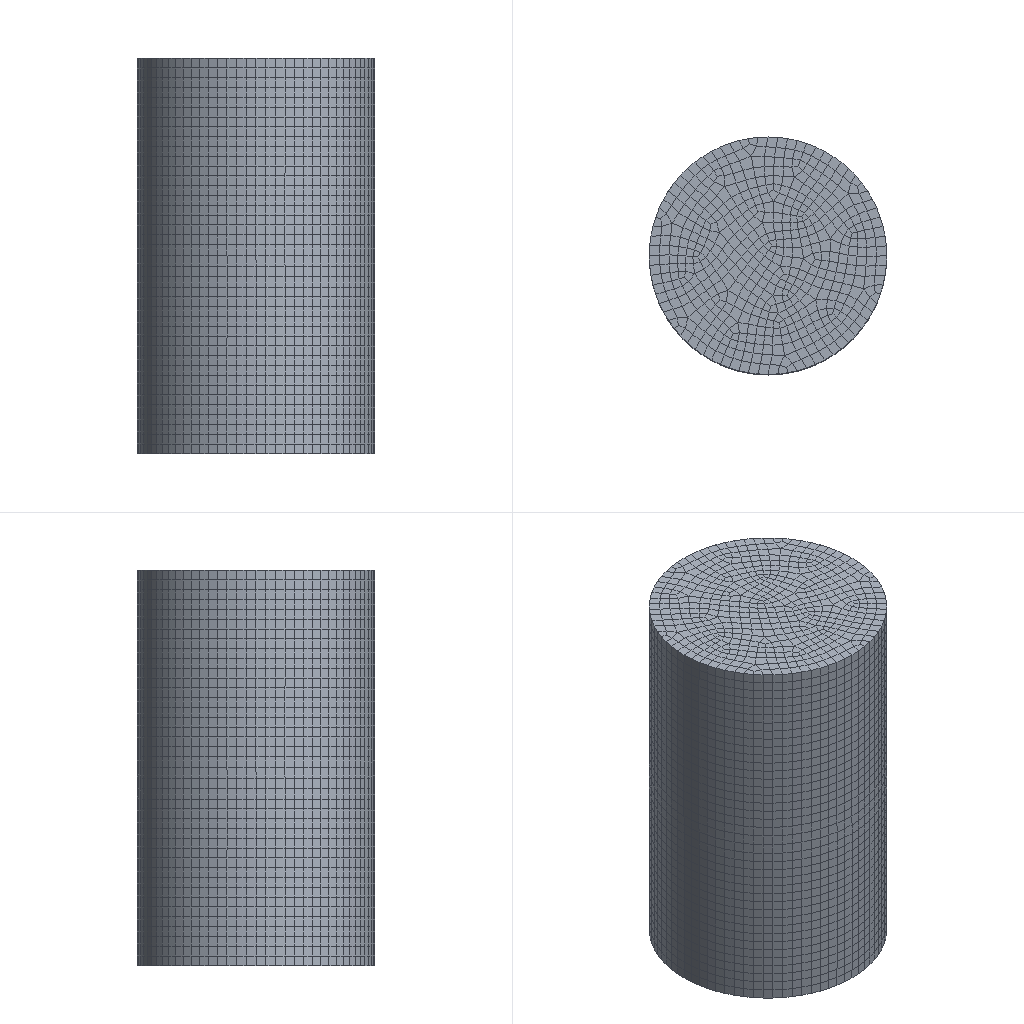Simulation study | ansys fluent
Set-up summary:
category,name,step,type,value,unit,region
solver,ansys_fluent,,Fluent 26.1.0
units,SI m-kg-s (Fluent internal),,stated,boundary values in the units shown in brackets; results in listed units
analysis,deck.cas,,cfd steady,"dimension=3D; solver=3d, dp, pbns, lam (3d, double precision, pressure-based, laminar); source_case=.cas"
model,Space,deck.cas,,3D
model,Time,deck.cas,,Steady
model,Viscous,deck.cas,,Laminar
model,Heat Transfer,deck.cas,,Enabled
model,Multiphase,deck.cas,,Disabled
mesh,nodes,,,23780
mesh,elements,,,21640
mesh,faces,,,66981
cell_zone,solid,deck.cas,solid,material=aluminum,,zone 2
material,air (fluid),,Density,1.225,kg/m^3
material,air (fluid),,Cp (Specific Heat),1006.43,J/(kg K)
material,air (fluid),,Thermal Conductivity,0.0242,W/(m K)
material,air (fluid),,Viscosity,1.7894e-05,kg/(m s)
material,aluminum (solid),,Density,2719,kg/m^3
material,aluminum (solid),,Cp (Specific Heat),871,J/(kg K)
material,aluminum (solid),,Thermal Conductivity,202.4,W/(m K)
bc,wall.down,deck.cas,wall,Material Name=aluminum; Thermal BC Type=Heat Flux,,zone 3
bc,wall.up,deck.cas,wall,Material Name=aluminum; Thermal BC Type=Heat Flux,,zone 4
bc,wall.out,deck.cas,wall,Material Name=aluminum; Thermal BC Type=Temperature; Temperature [K]=400,,zone 5
Results summary:
result,mass flow rate wall.down,deck.cas,,-0,kg/s
result,mass flow rate wall.out,deck.cas,,-0,kg/s
result,mass flow rate wall.up,deck.cas,,-0,kg/s
result,mass flow rate Net,deck.cas,,0,kg/s
result,heat transfer rate wall.down,deck.cas,,-0,W
result,heat transfer rate wall.out,deck.cas,,-180750,W
result,heat transfer rate wall.up,deck.cas,,-0,W
result,heat transfer rate Net,deck.cas,,-0.04312,W
result,wall force total wall.down,deck.cas,,"(0, 0, 0)",N
result,wall force pressure wall.down,deck.cas,,"(0, 0, 0)",N
result,wall force viscous wall.down,deck.cas,,"(0, 0, 0)",N
result,wall force total wall.out,deck.cas,,"(0, 0, 0)",N
result,wall force pressure wall.out,deck.cas,,"(0, 0, 0)",N
result,wall force viscous wall.out,deck.cas,,"(0, 0, 0)",N
result,wall force total wall.up,deck.cas,,"(0, 0, 0)",N
result,wall force pressure wall.up,deck.cas,,"(0, 0, 0)",N
result,wall force viscous wall.up,deck.cas,,"(0, 0, 0)",N
result,wall force total Net,deck.cas,,"(0, 0, 0)",N
result,wall force pressure Net,deck.cas,,"(0, 0, 0)",N
result,wall force viscous Net,deck.cas,,"(0, 0, 0)",N